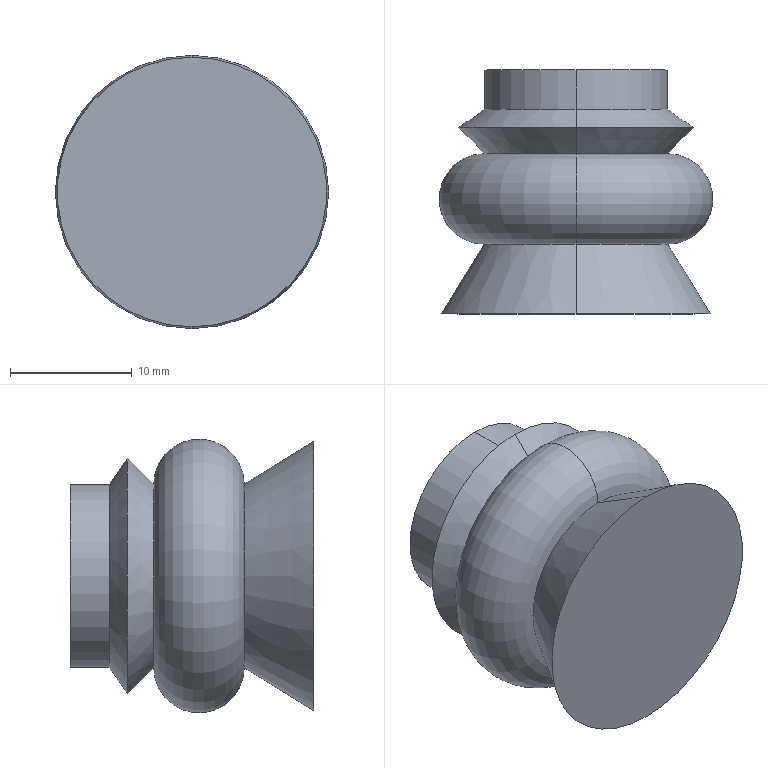Part | STEP file | 吸盘-2 | 1 solid | 12 faces | box 22.458 x 20 x 22.458 mm | volume 5536 mm3 | cone 6 | torus 2 | cylinder 2 | plane 2 | commonest cylinder face diameters 15 x2
STEP:
#1=CARTESIAN_POINT('',(0.,-11.893,7.53));
#2=VERTEX_POINT('',#1);
#3=CARTESIAN_POINT('',(0.,-11.893,-7.53));
#4=VERTEX_POINT('',#3);
#5=CARTESIAN_POINT('',(0.,-11.893,0.));
#6=DIRECTION('',(0.,1.,0.));
#7=DIRECTION('',(0.,0.,1.));
#8=AXIS2_PLACEMENT_3D('',#5,#6,#7);
#9=CIRCLE('',#8,7.53);
#10=EDGE_CURVE('',#2,#4,#9,.T.);
#11=ORIENTED_EDGE('',*,*,#10,.F.);
#12=CARTESIAN_POINT('',(0.,-17.604,11.045));
#13=VERTEX_POINT('',#12);
#14=CARTESIAN_POINT('',(0.,-17.604,11.045));
#15=DIRECTION('',(0.,-0.8517,0.5241));
#16=VECTOR('',#15,1000.);
#17=LINE('',#14,#16);
#18=EDGE_CURVE('',#2,#13,#17,.T.);
#19=ORIENTED_EDGE('',*,*,#18,.T.);
#20=CARTESIAN_POINT('',(0.,-17.604,-11.045));
#21=VERTEX_POINT('',#20);
#22=CARTESIAN_POINT('',(0.,-17.604,0.));
#23=DIRECTION('',(0.,1.,0.));
#24=DIRECTION('',(0.,0.,1.));
#25=AXIS2_PLACEMENT_3D('',#22,#23,#24);
#26=CIRCLE('',#25,11.045);
#27=EDGE_CURVE('',#13,#21,#26,.T.);
#28=ORIENTED_EDGE('',*,*,#27,.T.);
#29=CARTESIAN_POINT('',(0.,-17.604,-11.045));
#30=DIRECTION('',(0.,-0.8517,-0.5241));
#31=VECTOR('',#30,1000.);
#32=LINE('',#29,#31);
#33=EDGE_CURVE('',#4,#21,#32,.T.);
#34=ORIENTED_EDGE('',*,*,#33,.F.);
#35=EDGE_LOOP('',(#11,#19,#28,#34));
#36=FACE_OUTER_BOUND('',#35,.T.);
#37=CARTESIAN_POINT('',(0.,-17.604,0.));
#38=DIRECTION('',(0.,-1.,0.));
#39=DIRECTION('',(0.,0.,-1.));
#40=AXIS2_PLACEMENT_3D('',#37,#38,#39);
#41=CONICAL_SURFACE('',#40,11.045,0.5517);
#42=ADVANCED_FACE('',(#36),#41,.T.);
#43=ORIENTED_EDGE('',*,*,#10,.T.);
#44=CARTESIAN_POINT('',(0.,-4.466,-7.5));
#45=VERTEX_POINT('',#44);
#46=CARTESIAN_POINT('',(0.,-8.18,-7.515));
#47=DIRECTION('',(1.,0.,0.));
#48=DIRECTION('',(0.,0.,-1.));
#49=AXIS2_PLACEMENT_3D('',#46,#47,#48);
#50=CIRCLE('',#49,3.714);
#51=EDGE_CURVE('',#4,#45,#50,.T.);
#52=ORIENTED_EDGE('',*,*,#51,.T.);
#53=CARTESIAN_POINT('',(0.,-4.466,7.5));
#54=VERTEX_POINT('',#53);
#55=CARTESIAN_POINT('',(0.,-4.466,0.));
#56=DIRECTION('',(0.,1.,0.));
#57=DIRECTION('',(0.,0.,1.));
#58=AXIS2_PLACEMENT_3D('',#55,#56,#57);
#59=CIRCLE('',#58,7.5);
#60=EDGE_CURVE('',#54,#45,#59,.T.);
#61=ORIENTED_EDGE('',*,*,#60,.F.);
#62=CARTESIAN_POINT('',(0.,-8.18,7.515));
#63=DIRECTION('',(-1.,0.,0.));
#64=DIRECTION('',(0.,0.,1.));
#65=AXIS2_PLACEMENT_3D('',#62,#63,#64);
#66=CIRCLE('',#65,3.714);
#67=EDGE_CURVE('',#2,#54,#66,.T.);
#68=ORIENTED_EDGE('',*,*,#67,.F.);
#69=EDGE_LOOP('',(#43,#52,#61,#68));
#70=FACE_OUTER_BOUND('',#69,.T.);
#71=CARTESIAN_POINT('',(0.,-8.18,0.));
#72=DIRECTION('',(0.,1.,0.));
#73=DIRECTION('',(0.,0.,1.));
#74=AXIS2_PLACEMENT_3D('',#71,#72,#73);
#75=TOROIDAL_SURFACE('',#74,7.515,3.714);
#76=ADVANCED_FACE('',(#70),#75,.T.);
#77=ORIENTED_EDGE('',*,*,#60,.T.);
#78=CARTESIAN_POINT('',(0.,-2.312,-9.65));
#79=VERTEX_POINT('',#78);
#80=CARTESIAN_POINT('',(0.,-4.466,-7.5));
#81=DIRECTION('',(0.,0.7078,-0.7064));
#82=VECTOR('',#81,1000.);
#83=LINE('',#80,#82);
#84=EDGE_CURVE('',#45,#79,#83,.T.);
#85=ORIENTED_EDGE('',*,*,#84,.T.);
#86=CARTESIAN_POINT('',(0.,-2.312,9.65));
#87=VERTEX_POINT('',#86);
#88=CARTESIAN_POINT('',(0.,-2.312,0.));
#89=DIRECTION('',(0.,1.,0.));
#90=DIRECTION('',(0.,0.,1.));
#91=AXIS2_PLACEMENT_3D('',#88,#89,#90);
#92=CIRCLE('',#91,9.65);
#93=EDGE_CURVE('',#87,#79,#92,.T.);
#94=ORIENTED_EDGE('',*,*,#93,.F.);
#95=CARTESIAN_POINT('',(0.,-4.466,7.5));
#96=DIRECTION('',(0.,0.7078,0.7064));
#97=VECTOR('',#96,1000.);
#98=LINE('',#95,#97);
#99=EDGE_CURVE('',#54,#87,#98,.T.);
#100=ORIENTED_EDGE('',*,*,#99,.F.);
#101=EDGE_LOOP('',(#77,#85,#94,#100));
#102=FACE_OUTER_BOUND('',#101,.T.);
#103=CARTESIAN_POINT('',(0.,-4.466,0.));
#104=DIRECTION('',(0.,1.,0.));
#105=DIRECTION('',(0.,0.,1.));
#106=AXIS2_PLACEMENT_3D('',#103,#104,#105);
#107=CONICAL_SURFACE('',#106,7.5,0.7845);
#108=ADVANCED_FACE('',(#102),#107,.T.);
#109=CARTESIAN_POINT('',(0.,-0.8262,7.5));
#110=VERTEX_POINT('',#109);
#111=CARTESIAN_POINT('',(0.,-0.8262,-7.5));
#112=VERTEX_POINT('',#111);
#113=CARTESIAN_POINT('',(0.,-0.8262,0.));
#114=DIRECTION('',(0.,1.,0.));
#115=DIRECTION('',(0.,0.,1.));
#116=AXIS2_PLACEMENT_3D('',#113,#114,#115);
#117=CIRCLE('',#116,7.5);
#118=EDGE_CURVE('',#110,#112,#117,.T.);
#119=ORIENTED_EDGE('',*,*,#118,.F.);
#120=CARTESIAN_POINT('',(0.,-2.312,9.65));
#121=DIRECTION('',(0.,-0.5683,0.8228));
#122=VECTOR('',#121,1000.);
#123=LINE('',#120,#122);
#124=EDGE_CURVE('',#110,#87,#123,.T.);
#125=ORIENTED_EDGE('',*,*,#124,.T.);
#126=ORIENTED_EDGE('',*,*,#93,.T.);
#127=CARTESIAN_POINT('',(0.,-2.312,-9.65));
#128=DIRECTION('',(0.,-0.5683,-0.8228));
#129=VECTOR('',#128,1000.);
#130=LINE('',#127,#129);
#131=EDGE_CURVE('',#112,#79,#130,.T.);
#132=ORIENTED_EDGE('',*,*,#131,.F.);
#133=EDGE_LOOP('',(#119,#125,#126,#132));
#134=FACE_OUTER_BOUND('',#133,.T.);
#135=CARTESIAN_POINT('',(0.,-2.312,0.));
#136=DIRECTION('',(0.,-1.,0.));
#137=DIRECTION('',(0.,0.,-1.));
#138=AXIS2_PLACEMENT_3D('',#135,#136,#137);
#139=CONICAL_SURFACE('',#138,9.65,0.9663);
#140=ADVANCED_FACE('',(#134),#139,.T.);
#141=ORIENTED_EDGE('',*,*,#118,.T.);
#142=CARTESIAN_POINT('',(0.,2.396,-7.5));
#143=VERTEX_POINT('',#142);
#144=CARTESIAN_POINT('',(0.,33.934,-7.5));
#145=DIRECTION('',(0.,1.,0.));
#146=VECTOR('',#145,1000.);
#147=LINE('',#144,#146);
#148=EDGE_CURVE('',#112,#143,#147,.T.);
#149=ORIENTED_EDGE('',*,*,#148,.T.);
#150=CARTESIAN_POINT('',(0.,2.396,7.5));
#151=VERTEX_POINT('',#150);
#152=CARTESIAN_POINT('',(0.,2.396,0.));
#153=DIRECTION('',(0.,1.,0.));
#154=DIRECTION('',(0.,0.,1.));
#155=AXIS2_PLACEMENT_3D('',#152,#153,#154);
#156=CIRCLE('',#155,7.5);
#157=EDGE_CURVE('',#151,#143,#156,.T.);
#158=ORIENTED_EDGE('',*,*,#157,.F.);
#159=CARTESIAN_POINT('',(0.,33.934,7.5));
#160=DIRECTION('',(0.,1.,0.));
#161=VECTOR('',#160,1000.);
#162=LINE('',#159,#161);
#163=EDGE_CURVE('',#110,#151,#162,.T.);
#164=ORIENTED_EDGE('',*,*,#163,.F.);
#165=EDGE_LOOP('',(#141,#149,#158,#164));
#166=FACE_OUTER_BOUND('',#165,.T.);
#167=CARTESIAN_POINT('',(0.,33.934,0.));
#168=DIRECTION('',(0.,1.,0.));
#169=DIRECTION('',(0.,0.,1.));
#170=AXIS2_PLACEMENT_3D('',#167,#168,#169);
#171=CYLINDRICAL_SURFACE('',#170,7.5);
#172=ADVANCED_FACE('',(#166),#171,.T.);
#173=ORIENTED_EDGE('',*,*,#157,.T.);
#174=CARTESIAN_POINT('',(0.,2.396,0.));
#175=DIRECTION('',(0.,1.,0.));
#176=DIRECTION('',(0.,0.,1.));
#177=AXIS2_PLACEMENT_3D('',#174,#175,#176);
#178=CIRCLE('',#177,7.5);
#179=EDGE_CURVE('',#143,#151,#178,.T.);
#180=ORIENTED_EDGE('',*,*,#179,.T.);
#181=EDGE_LOOP('',(#173,#180));
#182=FACE_OUTER_BOUND('',#181,.T.);
#183=CARTESIAN_POINT('',(7.5,2.396,0.));
#184=DIRECTION('',(0.,-1.,0.));
#185=DIRECTION('',(0.,0.,-1.));
#186=AXIS2_PLACEMENT_3D('',#183,#184,#185);
#187=PLANE('',#186);
#188=ADVANCED_FACE('',(#182),#187,.F.);
#189=ORIENTED_EDGE('',*,*,#148,.F.);
#190=CARTESIAN_POINT('',(0.,-0.8262,0.));
#191=DIRECTION('',(0.,1.,0.));
#192=DIRECTION('',(0.,0.,1.));
#193=AXIS2_PLACEMENT_3D('',#190,#191,#192);
#194=CIRCLE('',#193,7.5);
#195=EDGE_CURVE('',#112,#110,#194,.T.);
#196=ORIENTED_EDGE('',*,*,#195,.T.);
#197=ORIENTED_EDGE('',*,*,#163,.T.);
#198=ORIENTED_EDGE('',*,*,#179,.F.);
#199=EDGE_LOOP('',(#189,#196,#197,#198));
#200=FACE_OUTER_BOUND('',#199,.T.);
#201=CARTESIAN_POINT('',(0.,33.934,0.));
#202=DIRECTION('',(0.,1.,0.));
#203=DIRECTION('',(0.,0.,1.));
#204=AXIS2_PLACEMENT_3D('',#201,#202,#203);
#205=CYLINDRICAL_SURFACE('',#204,7.5);
#206=ADVANCED_FACE('',(#200),#205,.T.);
#207=ORIENTED_EDGE('',*,*,#124,.F.);
#208=ORIENTED_EDGE('',*,*,#195,.F.);
#209=ORIENTED_EDGE('',*,*,#131,.T.);
#210=CARTESIAN_POINT('',(0.,-2.312,0.));
#211=DIRECTION('',(0.,1.,0.));
#212=DIRECTION('',(0.,0.,1.));
#213=AXIS2_PLACEMENT_3D('',#210,#211,#212);
#214=CIRCLE('',#213,9.65);
#215=EDGE_CURVE('',#79,#87,#214,.T.);
#216=ORIENTED_EDGE('',*,*,#215,.T.);
#217=EDGE_LOOP('',(#207,#208,#209,#216));
#218=FACE_OUTER_BOUND('',#217,.T.);
#219=CARTESIAN_POINT('',(0.,-2.312,0.));
#220=DIRECTION('',(0.,-1.,0.));
#221=DIRECTION('',(0.,0.,-1.));
#222=AXIS2_PLACEMENT_3D('',#219,#220,#221);
#223=CONICAL_SURFACE('',#222,9.65,0.9663);
#224=ADVANCED_FACE('',(#218),#223,.T.);
#225=ORIENTED_EDGE('',*,*,#84,.F.);
#226=CARTESIAN_POINT('',(0.,-4.466,0.));
#227=DIRECTION('',(0.,1.,0.));
#228=DIRECTION('',(0.,0.,1.));
#229=AXIS2_PLACEMENT_3D('',#226,#227,#228);
#230=CIRCLE('',#229,7.5);
#231=EDGE_CURVE('',#45,#54,#230,.T.);
#232=ORIENTED_EDGE('',*,*,#231,.T.);
#233=ORIENTED_EDGE('',*,*,#99,.T.);
#234=ORIENTED_EDGE('',*,*,#215,.F.);
#235=EDGE_LOOP('',(#225,#232,#233,#234));
#236=FACE_OUTER_BOUND('',#235,.T.);
#237=CARTESIAN_POINT('',(0.,-4.466,0.));
#238=DIRECTION('',(0.,1.,0.));
#239=DIRECTION('',(0.,0.,1.));
#240=AXIS2_PLACEMENT_3D('',#237,#238,#239);
#241=CONICAL_SURFACE('',#240,7.5,0.7845);
#242=ADVANCED_FACE('',(#236),#241,.T.);
#243=ORIENTED_EDGE('',*,*,#51,.F.);
#244=CARTESIAN_POINT('',(0.,-11.893,0.));
#245=DIRECTION('',(0.,1.,0.));
#246=DIRECTION('',(0.,0.,1.));
#247=AXIS2_PLACEMENT_3D('',#244,#245,#246);
#248=CIRCLE('',#247,7.53);
#249=EDGE_CURVE('',#4,#2,#248,.T.);
#250=ORIENTED_EDGE('',*,*,#249,.T.);
#251=ORIENTED_EDGE('',*,*,#67,.T.);
#252=ORIENTED_EDGE('',*,*,#231,.F.);
#253=EDGE_LOOP('',(#243,#250,#251,#252));
#254=FACE_OUTER_BOUND('',#253,.T.);
#255=CARTESIAN_POINT('',(0.,-8.18,0.));
#256=DIRECTION('',(0.,1.,0.));
#257=DIRECTION('',(0.,0.,1.));
#258=AXIS2_PLACEMENT_3D('',#255,#256,#257);
#259=TOROIDAL_SURFACE('',#258,7.515,3.714);
#260=ADVANCED_FACE('',(#254),#259,.T.);
#261=ORIENTED_EDGE('',*,*,#18,.F.);
#262=ORIENTED_EDGE('',*,*,#249,.F.);
#263=ORIENTED_EDGE('',*,*,#33,.T.);
#264=CARTESIAN_POINT('',(0.,-17.604,0.));
#265=DIRECTION('',(0.,1.,0.));
#266=DIRECTION('',(0.,0.,1.));
#267=AXIS2_PLACEMENT_3D('',#264,#265,#266);
#268=CIRCLE('',#267,11.045);
#269=EDGE_CURVE('',#21,#13,#268,.T.);
#270=ORIENTED_EDGE('',*,*,#269,.T.);
#271=EDGE_LOOP('',(#261,#262,#263,#270));
#272=FACE_OUTER_BOUND('',#271,.T.);
#273=CARTESIAN_POINT('',(0.,-17.604,0.));
#274=DIRECTION('',(0.,-1.,0.));
#275=DIRECTION('',(0.,0.,-1.));
#276=AXIS2_PLACEMENT_3D('',#273,#274,#275);
#277=CONICAL_SURFACE('',#276,11.045,0.5517);
#278=ADVANCED_FACE('',(#272),#277,.T.);
#279=ORIENTED_EDGE('',*,*,#269,.F.);
#280=ORIENTED_EDGE('',*,*,#27,.F.);
#281=EDGE_LOOP('',(#279,#280));
#282=FACE_OUTER_BOUND('',#281,.T.);
#283=CARTESIAN_POINT('',(0.,-17.604,0.));
#284=DIRECTION('',(0.,1.,0.));
#285=DIRECTION('',(0.,0.,1.));
#286=AXIS2_PLACEMENT_3D('',#283,#284,#285);
#287=PLANE('',#286);
#288=ADVANCED_FACE('',(#282),#287,.F.);
#289=CLOSED_SHELL('',(#42,#76,#108,#140,#172,#188,#206,#224,#242,#260,#278,#288));
#290=MANIFOLD_SOLID_BREP('',#289);
#291=CARTESIAN_POINT('',(0.,0.,0.));
#292=DIRECTION('',(0.,0.,1.));
#293=DIRECTION('',(1.,0.,0.));
#294=AXIS2_PLACEMENT_3D('',#291,#292,#293);
#295=(LENGTH_UNIT()NAMED_UNIT(*)SI_UNIT(.MILLI.,.METRE.));
#296=UNCERTAINTY_MEASURE_WITH_UNIT(LENGTH_MEASURE(0.00001),#295,'','');
#297=(NAMED_UNIT(*)PLANE_ANGLE_UNIT()SI_UNIT($,.RADIAN.));
#298=(NAMED_UNIT(*)SI_UNIT($,.STERADIAN.)SOLID_ANGLE_UNIT());
#299=(GEOMETRIC_REPRESENTATION_CONTEXT(3)GLOBAL_UNCERTAINTY_ASSIGNED_CONTEXT((#296))GLOBAL_UNIT_ASSIGNED_CONTEXT((#295,#297,#298))REPRESENTATION_CONTEXT('',''));
#300=ADVANCED_BREP_SHAPE_REPRESENTATION('',(#290,#294),#299);